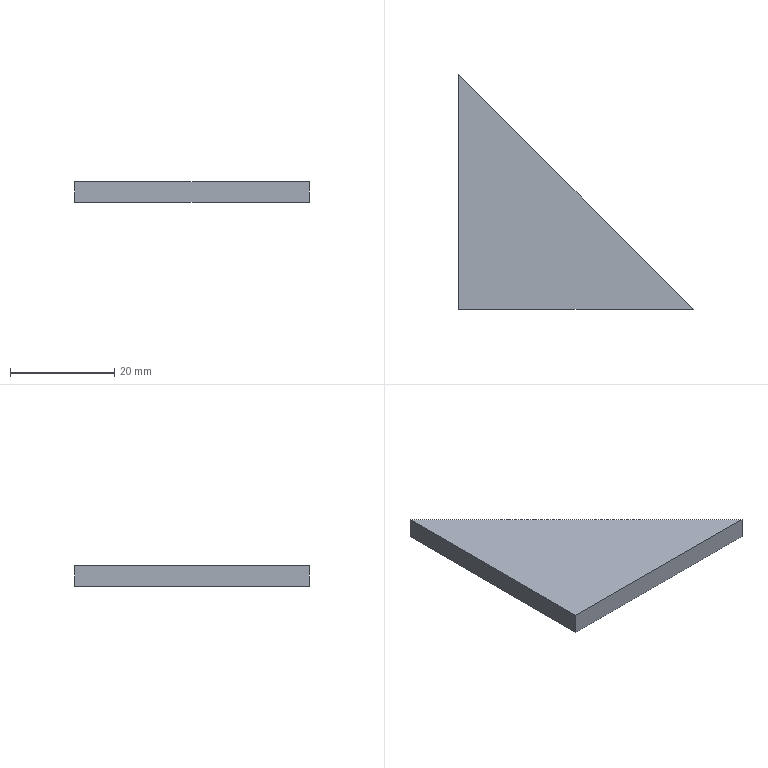Part | STEP file | Q7C0517 | 1 solid | 5 faces | box 45 x 45 x 4 mm | volume 4050 mm3 | plane 5
STEP:
#1=CARTESIAN_POINT('',(0.,0.,0.));
#2=DIRECTION('',(0.,0.,1.));
#3=DIRECTION('',(1.,0.,0.));
#4=AXIS2_PLACEMENT_3D('',#1,#2,#3);
#5=CARTESIAN_POINT('',(0.,0.,0.));
#6=VERTEX_POINT('',#5);
#7=CARTESIAN_POINT('',(45.,0.,0.));
#8=VERTEX_POINT('',#7);
#9=CARTESIAN_POINT('',(45.,0.,0.));
#10=DIRECTION('',(1.,0.,0.));
#11=VECTOR('',#10,1.);
#12=LINE('',#9,#11);
#13=CARTESIAN_POINT('',(45.,0.,4.));
#14=DIRECTION('',(0.,1.,0.));
#15=DIRECTION('',(-1.,0.,0.));
#16=AXIS2_PLACEMENT_3D('',#13,#14,#15);
#17=PLANE('',#16);
#18=CARTESIAN_POINT('',(0.,-4.));
#19=DIRECTION('',(-1.,0.));
#20=VECTOR('',#19,1.);
#21=LINE('',#18,#20);
#22=(GEOMETRIC_REPRESENTATION_CONTEXT(2)PARAMETRIC_REPRESENTATION_CONTEXT()REPRESENTATION_CONTEXT('',''));
#23=DEFINITIONAL_REPRESENTATION('',(#21),#22);
#24=PCURVE('',#17,#23);
#25=CARTESIAN_POINT('',(0.,0.,0.));
#26=DIRECTION('',(0.,0.,-1.));
#27=DIRECTION('',(-1.,0.,0.));
#28=AXIS2_PLACEMENT_3D('',#25,#26,#27);
#29=PLANE('',#28);
#30=CARTESIAN_POINT('',(-45.,0.));
#31=DIRECTION('',(-1.,0.));
#32=VECTOR('',#31,1.);
#33=LINE('',#30,#32);
#34=(GEOMETRIC_REPRESENTATION_CONTEXT(2)PARAMETRIC_REPRESENTATION_CONTEXT()REPRESENTATION_CONTEXT('',''));
#35=DEFINITIONAL_REPRESENTATION('',(#33),#34);
#36=PCURVE('',#29,#35);
#37=SURFACE_CURVE('',#12,(#24,#36),.PCURVE_S1.);
#38=EDGE_CURVE('',#6,#8,#37,.T.);
#39=ORIENTED_EDGE('',*,*,#38,.T.);
#40=CARTESIAN_POINT('',(45.,0.,4.));
#41=VERTEX_POINT('',#40);
#42=CARTESIAN_POINT('',(45.,0.,4.));
#43=DIRECTION('',(0.,0.,-1.));
#44=VECTOR('',#43,1.);
#45=LINE('',#42,#44);
#46=CARTESIAN_POINT('',(0.,0.));
#47=DIRECTION('',(0.,-1.));
#48=VECTOR('',#47,1.);
#49=LINE('',#46,#48);
#50=(GEOMETRIC_REPRESENTATION_CONTEXT(2)PARAMETRIC_REPRESENTATION_CONTEXT()REPRESENTATION_CONTEXT('',''));
#51=DEFINITIONAL_REPRESENTATION('',(#49),#50);
#52=PCURVE('',#17,#51);
#53=CARTESIAN_POINT('',(0.,45.,4.));
#54=DIRECTION('',(-0.7071,-0.7071,0.));
#55=DIRECTION('',(0.7071,-0.7071,0.));
#56=AXIS2_PLACEMENT_3D('',#53,#54,#55);
#57=PLANE('',#56);
#58=CARTESIAN_POINT('',(63.64,0.));
#59=DIRECTION('',(0.,-1.));
#60=VECTOR('',#59,1.);
#61=LINE('',#58,#60);
#62=(GEOMETRIC_REPRESENTATION_CONTEXT(2)PARAMETRIC_REPRESENTATION_CONTEXT()REPRESENTATION_CONTEXT('',''));
#63=DEFINITIONAL_REPRESENTATION('',(#61),#62);
#64=PCURVE('',#57,#63);
#65=SURFACE_CURVE('',#45,(#52,#64),.PCURVE_S1.);
#66=EDGE_CURVE('',#41,#8,#65,.T.);
#67=ORIENTED_EDGE('',*,*,#66,.F.);
#68=CARTESIAN_POINT('',(0.,0.,4.));
#69=VERTEX_POINT('',#68);
#70=CARTESIAN_POINT('',(45.,0.,4.));
#71=DIRECTION('',(1.,0.,0.));
#72=VECTOR('',#71,1.);
#73=LINE('',#70,#72);
#74=CARTESIAN_POINT('',(0.,0.));
#75=DIRECTION('',(-1.,0.));
#76=VECTOR('',#75,1.);
#77=LINE('',#74,#76);
#78=(GEOMETRIC_REPRESENTATION_CONTEXT(2)PARAMETRIC_REPRESENTATION_CONTEXT()REPRESENTATION_CONTEXT('',''));
#79=DEFINITIONAL_REPRESENTATION('',(#77),#78);
#80=PCURVE('',#17,#79);
#81=CARTESIAN_POINT('',(0.,0.,4.));
#82=DIRECTION('',(0.,0.,-1.));
#83=DIRECTION('',(-1.,0.,0.));
#84=AXIS2_PLACEMENT_3D('',#81,#82,#83);
#85=PLANE('',#84);
#86=CARTESIAN_POINT('',(-45.,0.));
#87=DIRECTION('',(-1.,0.));
#88=VECTOR('',#87,1.);
#89=LINE('',#86,#88);
#90=(GEOMETRIC_REPRESENTATION_CONTEXT(2)PARAMETRIC_REPRESENTATION_CONTEXT()REPRESENTATION_CONTEXT('',''));
#91=DEFINITIONAL_REPRESENTATION('',(#89),#90);
#92=PCURVE('',#85,#91);
#93=SURFACE_CURVE('',#73,(#80,#92),.PCURVE_S1.);
#94=EDGE_CURVE('',#69,#41,#93,.T.);
#95=ORIENTED_EDGE('',*,*,#94,.F.);
#96=CARTESIAN_POINT('',(0.,0.,4.));
#97=DIRECTION('',(0.,0.,-1.));
#98=VECTOR('',#97,1.);
#99=LINE('',#96,#98);
#100=CARTESIAN_POINT('',(45.,0.));
#101=DIRECTION('',(0.,-1.));
#102=VECTOR('',#101,1.);
#103=LINE('',#100,#102);
#104=(GEOMETRIC_REPRESENTATION_CONTEXT(2)PARAMETRIC_REPRESENTATION_CONTEXT()REPRESENTATION_CONTEXT('',''));
#105=DEFINITIONAL_REPRESENTATION('',(#103),#104);
#106=PCURVE('',#17,#105);
#107=CARTESIAN_POINT('',(0.,0.,4.));
#108=DIRECTION('',(1.,0.,0.));
#109=DIRECTION('',(0.,0.,-1.));
#110=AXIS2_PLACEMENT_3D('',#107,#108,#109);
#111=PLANE('',#110);
#112=CARTESIAN_POINT('',(0.,0.));
#113=DIRECTION('',(1.,0.));
#114=VECTOR('',#113,1.);
#115=LINE('',#112,#114);
#116=(GEOMETRIC_REPRESENTATION_CONTEXT(2)PARAMETRIC_REPRESENTATION_CONTEXT()REPRESENTATION_CONTEXT('',''));
#117=DEFINITIONAL_REPRESENTATION('',(#115),#116);
#118=PCURVE('',#111,#117);
#119=SURFACE_CURVE('',#99,(#106,#118),.PCURVE_S1.);
#120=EDGE_CURVE('',#69,#6,#119,.T.);
#121=ORIENTED_EDGE('',*,*,#120,.T.);
#122=EDGE_LOOP('',(#39,#67,#95,#121));
#123=FACE_BOUND('',#122,.T.);
#124=ADVANCED_FACE('',(#123),#17,.F.);
#125=CARTESIAN_POINT('',(0.,45.,0.));
#126=VERTEX_POINT('',#125);
#127=CARTESIAN_POINT('',(0.,45.,0.));
#128=DIRECTION('',(-0.7071,0.7071,0.));
#129=VECTOR('',#128,1.);
#130=LINE('',#127,#129);
#131=CARTESIAN_POINT('',(0.,-4.));
#132=DIRECTION('',(-1.,0.));
#133=VECTOR('',#132,1.);
#134=LINE('',#131,#133);
#135=(GEOMETRIC_REPRESENTATION_CONTEXT(2)PARAMETRIC_REPRESENTATION_CONTEXT()REPRESENTATION_CONTEXT('',''));
#136=DEFINITIONAL_REPRESENTATION('',(#134),#135);
#137=PCURVE('',#57,#136);
#138=CARTESIAN_POINT('',(0.,45.));
#139=DIRECTION('',(0.7071,0.7071));
#140=VECTOR('',#139,1.);
#141=LINE('',#138,#140);
#142=(GEOMETRIC_REPRESENTATION_CONTEXT(2)PARAMETRIC_REPRESENTATION_CONTEXT()REPRESENTATION_CONTEXT('',''));
#143=DEFINITIONAL_REPRESENTATION('',(#141),#142);
#144=PCURVE('',#29,#143);
#145=SURFACE_CURVE('',#130,(#137,#144),.PCURVE_S1.);
#146=EDGE_CURVE('',#8,#126,#145,.T.);
#147=ORIENTED_EDGE('',*,*,#146,.T.);
#148=CARTESIAN_POINT('',(0.,45.,4.));
#149=VERTEX_POINT('',#148);
#150=CARTESIAN_POINT('',(0.,45.,4.));
#151=DIRECTION('',(0.,0.,-1.));
#152=VECTOR('',#151,1.);
#153=LINE('',#150,#152);
#154=CARTESIAN_POINT('',(0.,0.));
#155=DIRECTION('',(0.,-1.));
#156=VECTOR('',#155,1.);
#157=LINE('',#154,#156);
#158=(GEOMETRIC_REPRESENTATION_CONTEXT(2)PARAMETRIC_REPRESENTATION_CONTEXT()REPRESENTATION_CONTEXT('',''));
#159=DEFINITIONAL_REPRESENTATION('',(#157),#158);
#160=PCURVE('',#57,#159);
#161=CARTESIAN_POINT('',(0.,45.));
#162=DIRECTION('',(1.,0.));
#163=VECTOR('',#162,1.);
#164=LINE('',#161,#163);
#165=(GEOMETRIC_REPRESENTATION_CONTEXT(2)PARAMETRIC_REPRESENTATION_CONTEXT()REPRESENTATION_CONTEXT('',''));
#166=DEFINITIONAL_REPRESENTATION('',(#164),#165);
#167=PCURVE('',#111,#166);
#168=SURFACE_CURVE('',#153,(#160,#167),.PCURVE_S1.);
#169=EDGE_CURVE('',#149,#126,#168,.T.);
#170=ORIENTED_EDGE('',*,*,#169,.F.);
#171=CARTESIAN_POINT('',(0.,45.,4.));
#172=DIRECTION('',(-0.7071,0.7071,0.));
#173=VECTOR('',#172,1.);
#174=LINE('',#171,#173);
#175=CARTESIAN_POINT('',(0.,0.));
#176=DIRECTION('',(-1.,0.));
#177=VECTOR('',#176,1.);
#178=LINE('',#175,#177);
#179=(GEOMETRIC_REPRESENTATION_CONTEXT(2)PARAMETRIC_REPRESENTATION_CONTEXT()REPRESENTATION_CONTEXT('',''));
#180=DEFINITIONAL_REPRESENTATION('',(#178),#179);
#181=PCURVE('',#57,#180);
#182=CARTESIAN_POINT('',(0.,45.));
#183=DIRECTION('',(0.7071,0.7071));
#184=VECTOR('',#183,1.);
#185=LINE('',#182,#184);
#186=(GEOMETRIC_REPRESENTATION_CONTEXT(2)PARAMETRIC_REPRESENTATION_CONTEXT()REPRESENTATION_CONTEXT('',''));
#187=DEFINITIONAL_REPRESENTATION('',(#185),#186);
#188=PCURVE('',#85,#187);
#189=SURFACE_CURVE('',#174,(#181,#188),.PCURVE_S1.);
#190=EDGE_CURVE('',#41,#149,#189,.T.);
#191=ORIENTED_EDGE('',*,*,#190,.F.);
#192=ORIENTED_EDGE('',*,*,#66,.T.);
#193=EDGE_LOOP('',(#147,#170,#191,#192));
#194=FACE_BOUND('',#193,.T.);
#195=ADVANCED_FACE('',(#194),#57,.F.);
#196=CARTESIAN_POINT('',(0.,0.,0.));
#197=DIRECTION('',(0.,-1.,0.));
#198=VECTOR('',#197,1.);
#199=LINE('',#196,#198);
#200=CARTESIAN_POINT('',(4.,0.));
#201=DIRECTION('',(0.,-1.));
#202=VECTOR('',#201,1.);
#203=LINE('',#200,#202);
#204=(GEOMETRIC_REPRESENTATION_CONTEXT(2)PARAMETRIC_REPRESENTATION_CONTEXT()REPRESENTATION_CONTEXT('',''));
#205=DEFINITIONAL_REPRESENTATION('',(#203),#204);
#206=PCURVE('',#111,#205);
#207=CARTESIAN_POINT('',(0.,0.));
#208=DIRECTION('',(0.,-1.));
#209=VECTOR('',#208,1.);
#210=LINE('',#207,#209);
#211=(GEOMETRIC_REPRESENTATION_CONTEXT(2)PARAMETRIC_REPRESENTATION_CONTEXT()REPRESENTATION_CONTEXT('',''));
#212=DEFINITIONAL_REPRESENTATION('',(#210),#211);
#213=PCURVE('',#29,#212);
#214=SURFACE_CURVE('',#199,(#206,#213),.PCURVE_S1.);
#215=EDGE_CURVE('',#126,#6,#214,.T.);
#216=ORIENTED_EDGE('',*,*,#215,.T.);
#217=ORIENTED_EDGE('',*,*,#120,.F.);
#218=CARTESIAN_POINT('',(0.,0.,4.));
#219=DIRECTION('',(0.,-1.,0.));
#220=VECTOR('',#219,1.);
#221=LINE('',#218,#220);
#222=CARTESIAN_POINT('',(0.,0.));
#223=DIRECTION('',(0.,-1.));
#224=VECTOR('',#223,1.);
#225=LINE('',#222,#224);
#226=(GEOMETRIC_REPRESENTATION_CONTEXT(2)PARAMETRIC_REPRESENTATION_CONTEXT()REPRESENTATION_CONTEXT('',''));
#227=DEFINITIONAL_REPRESENTATION('',(#225),#226);
#228=PCURVE('',#111,#227);
#229=CARTESIAN_POINT('',(0.,0.));
#230=DIRECTION('',(0.,-1.));
#231=VECTOR('',#230,1.);
#232=LINE('',#229,#231);
#233=(GEOMETRIC_REPRESENTATION_CONTEXT(2)PARAMETRIC_REPRESENTATION_CONTEXT()REPRESENTATION_CONTEXT('',''));
#234=DEFINITIONAL_REPRESENTATION('',(#232),#233);
#235=PCURVE('',#85,#234);
#236=SURFACE_CURVE('',#221,(#228,#235),.PCURVE_S1.);
#237=EDGE_CURVE('',#149,#69,#236,.T.);
#238=ORIENTED_EDGE('',*,*,#237,.F.);
#239=ORIENTED_EDGE('',*,*,#169,.T.);
#240=EDGE_LOOP('',(#216,#217,#238,#239));
#241=FACE_BOUND('',#240,.T.);
#242=ADVANCED_FACE('',(#241),#111,.F.);
#243=ORIENTED_EDGE('',*,*,#94,.T.);
#244=ORIENTED_EDGE('',*,*,#190,.T.);
#245=ORIENTED_EDGE('',*,*,#237,.T.);
#246=EDGE_LOOP('',(#243,#244,#245));
#247=FACE_BOUND('',#246,.T.);
#248=ADVANCED_FACE('',(#247),#85,.F.);
#249=ORIENTED_EDGE('',*,*,#38,.F.);
#250=ORIENTED_EDGE('',*,*,#215,.F.);
#251=ORIENTED_EDGE('',*,*,#146,.F.);
#252=EDGE_LOOP('',(#249,#250,#251));
#253=FACE_BOUND('',#252,.T.);
#254=ADVANCED_FACE('',(#253),#29,.T.);
#255=CLOSED_SHELL('',(#124,#195,#242,#248,#254));
#256=MANIFOLD_SOLID_BREP('',#255);
#257=(LENGTH_UNIT()NAMED_UNIT(*)SI_UNIT(.MILLI.,.METRE.));
#258=UNCERTAINTY_MEASURE_WITH_UNIT(LENGTH_MEASURE(0.0000001),#257,'','');
#259=(NAMED_UNIT(*)PLANE_ANGLE_UNIT()SI_UNIT($,.RADIAN.));
#260=(NAMED_UNIT(*)SI_UNIT($,.STERADIAN.)SOLID_ANGLE_UNIT());
#261=(GEOMETRIC_REPRESENTATION_CONTEXT(3)GLOBAL_UNCERTAINTY_ASSIGNED_CONTEXT((#258))GLOBAL_UNIT_ASSIGNED_CONTEXT((#257,#259,#260))REPRESENTATION_CONTEXT('',''));
#262=ADVANCED_BREP_SHAPE_REPRESENTATION('',(#4,#256),#261);